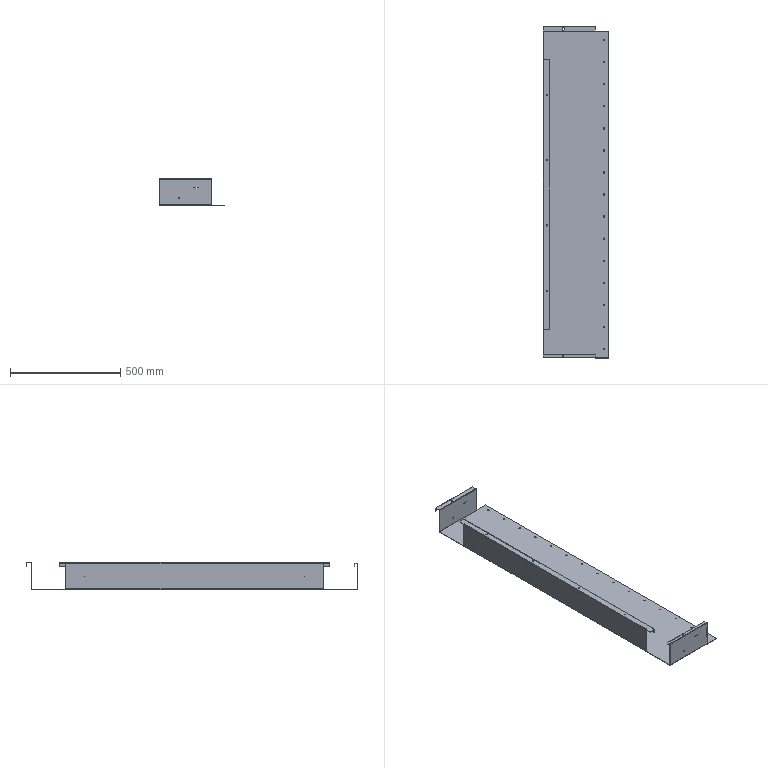Part | STEP file | SX-004-04 | 1 solid | 156 faces | box 295.5 x 1503 x 122 mm | volume 1401586 mm3 | plane 88 | cylinder 68 | commonest cylinder face diameters 7 x30 5.4 x14 0.4 x9 4.4 x9 3 x4 8 x2